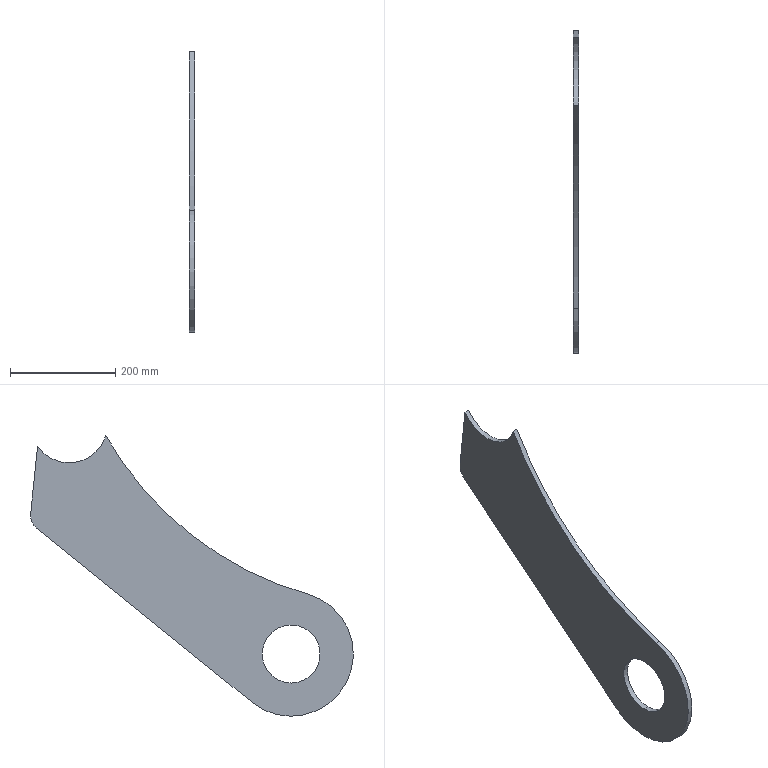Part | SolidWorks | features Extrusion 1 | 1 solid | 10 faces | box 10 x 612.332 x 532.004 mm | volume 1222648 mm3 | cylinder 6 | plane 4 | commonest cylinder face diameters 110 x2 60 x1 146 x1 236.039 x1 1284 x1
STEP:
#1=CARTESIAN_POINT('',(10.,206.6,-676.4));
#2=VERTEX_POINT('',#1);
#3=CARTESIAN_POINT('',(10.,206.6,-786.4));
#4=VERTEX_POINT('',#3);
#5=CARTESIAN_POINT('',(10.,206.6,-731.4));
#6=DIRECTION('',(1.,0.,0.));
#7=DIRECTION('',(0.,0.,-1.));
#8=AXIS2_PLACEMENT_3D('',#5,#6,#7);
#9=CIRCLE('',#8,55.);
#10=EDGE_CURVE('',#2,#4,#9,.T.);
#11=ORIENTED_EDGE('',*,*,#10,.T.);
#12=CARTESIAN_POINT('',(0.,206.6,-786.4));
#13=VERTEX_POINT('',#12);
#14=CARTESIAN_POINT('',(10.,206.6,-786.4));
#15=DIRECTION('',(-1.,0.,0.));
#16=VECTOR('',#15,1000.);
#17=LINE('',#14,#16);
#18=EDGE_CURVE('',#4,#13,#17,.T.);
#19=ORIENTED_EDGE('',*,*,#18,.T.);
#20=CARTESIAN_POINT('',(0.,206.6,-676.4));
#21=VERTEX_POINT('',#20);
#22=CARTESIAN_POINT('',(0.,206.6,-731.4));
#23=DIRECTION('',(1.,0.,0.));
#24=DIRECTION('',(0.,0.,-1.));
#25=AXIS2_PLACEMENT_3D('',#22,#23,#24);
#26=CIRCLE('',#25,55.);
#27=EDGE_CURVE('',#21,#13,#26,.T.);
#28=ORIENTED_EDGE('',*,*,#27,.F.);
#29=CARTESIAN_POINT('',(10.,206.6,-676.4));
#30=DIRECTION('',(-1.,0.,0.));
#31=VECTOR('',#30,1000.);
#32=LINE('',#29,#31);
#33=EDGE_CURVE('',#2,#21,#32,.T.);
#34=ORIENTED_EDGE('',*,*,#33,.F.);
#35=EDGE_LOOP('',(#11,#19,#28,#34));
#36=FACE_OUTER_BOUND('',#35,.T.);
#37=CARTESIAN_POINT('',(10.,206.6,-731.4));
#38=DIRECTION('',(-1.,0.,0.));
#39=DIRECTION('',(0.,0.,1.));
#40=AXIS2_PLACEMENT_3D('',#37,#38,#39);
#41=CYLINDRICAL_SURFACE('',#40,55.);
#42=ADVANCED_FACE('',(#36),#41,.F.);
#43=CARTESIAN_POINT('',(10.,687.7,-337.625));
#44=VERTEX_POINT('',#43);
#45=CARTESIAN_POINT('',(10.,558.043,-317.415));
#46=VERTEX_POINT('',#45);
#47=CARTESIAN_POINT('',(10.,627.8,-295.9));
#48=DIRECTION('',(-1.,0.,0.));
#49=DIRECTION('',(0.,0.,-1.));
#50=AXIS2_PLACEMENT_3D('',#47,#48,#49);
#51=CIRCLE('',#50,73.);
#52=EDGE_CURVE('',#44,#46,#51,.T.);
#53=ORIENTED_EDGE('',*,*,#52,.T.);
#54=CARTESIAN_POINT('',(10.,174.518,-617.825));
#55=VERTEX_POINT('',#54);
#56=CARTESIAN_POINT('',(10.,0.,0.));
#57=DIRECTION('',(-1.,0.,0.));
#58=DIRECTION('',(0.,0.,-1.));
#59=AXIS2_PLACEMENT_3D('',#56,#57,#58);
#60=CIRCLE('',#59,642.);
#61=EDGE_CURVE('',#46,#55,#60,.T.);
#62=ORIENTED_EDGE('',*,*,#61,.T.);
#63=CARTESIAN_POINT('',(10.,280.803,-823.175));
#64=VERTEX_POINT('',#63);
#65=CARTESIAN_POINT('',(10.,206.6,-731.4));
#66=DIRECTION('',(1.,0.,0.));
#67=DIRECTION('',(0.,0.,-1.));
#68=AXIS2_PLACEMENT_3D('',#65,#66,#67);
#69=CIRCLE('',#68,118.019);
#70=EDGE_CURVE('',#55,#64,#69,.T.);
#71=ORIENTED_EDGE('',*,*,#70,.T.);
#72=CARTESIAN_POINT('',(10.,689.774,-492.508));
#73=VERTEX_POINT('',#72);
#74=CARTESIAN_POINT('',(10.,689.774,-492.508));
#75=DIRECTION('',(0.,0.7776,0.6287));
#76=VECTOR('',#75,1000.);
#77=LINE('',#74,#76);
#78=EDGE_CURVE('',#64,#73,#77,.T.);
#79=ORIENTED_EDGE('',*,*,#78,.T.);
#80=CARTESIAN_POINT('',(10.,700.759,-466.147));
#81=VERTEX_POINT('',#80);
#82=CARTESIAN_POINT('',(10.,670.912,-469.18));
#83=DIRECTION('',(1.,0.,0.));
#84=DIRECTION('',(0.,0.,1.));
#85=AXIS2_PLACEMENT_3D('',#82,#83,#84);
#86=CIRCLE('',#85,30.);
#87=EDGE_CURVE('',#73,#81,#86,.T.);
#88=ORIENTED_EDGE('',*,*,#87,.T.);
#89=CARTESIAN_POINT('',(10.,687.7,-337.625));
#90=DIRECTION('',(0.,-0.1011,0.9949));
#91=VECTOR('',#90,1000.);
#92=LINE('',#89,#91);
#93=EDGE_CURVE('',#81,#44,#92,.T.);
#94=ORIENTED_EDGE('',*,*,#93,.T.);
#95=EDGE_LOOP('',(#53,#62,#71,#79,#88,#94));
#96=FACE_OUTER_BOUND('',#95,.T.);
#97=ORIENTED_EDGE('',*,*,#10,.F.);
#98=CARTESIAN_POINT('',(10.,206.6,-731.4));
#99=DIRECTION('',(1.,0.,0.));
#100=DIRECTION('',(0.,0.,-1.));
#101=AXIS2_PLACEMENT_3D('',#98,#99,#100);
#102=CIRCLE('',#101,55.);
#103=EDGE_CURVE('',#4,#2,#102,.T.);
#104=ORIENTED_EDGE('',*,*,#103,.F.);
#105=EDGE_LOOP('',(#97,#104));
#106=FACE_BOUND('',#105,.T.);
#107=CARTESIAN_POINT('',(10.,627.8,-295.9));
#108=DIRECTION('',(1.,0.,0.));
#109=DIRECTION('',(0.,0.,-1.));
#110=AXIS2_PLACEMENT_3D('',#107,#108,#109);
#111=PLANE('',#110);
#112=ADVANCED_FACE('',(#96,#106),#111,.T.);
#113=CARTESIAN_POINT('',(0.,687.7,-337.625));
#114=VERTEX_POINT('',#113);
#115=CARTESIAN_POINT('',(0.,558.043,-317.415));
#116=VERTEX_POINT('',#115);
#117=CARTESIAN_POINT('',(0.,627.8,-295.9));
#118=DIRECTION('',(-1.,0.,0.));
#119=DIRECTION('',(0.,0.,-1.));
#120=AXIS2_PLACEMENT_3D('',#117,#118,#119);
#121=CIRCLE('',#120,73.);
#122=EDGE_CURVE('',#114,#116,#121,.T.);
#123=ORIENTED_EDGE('',*,*,#122,.F.);
#124=CARTESIAN_POINT('',(0.,700.759,-466.147));
#125=VERTEX_POINT('',#124);
#126=CARTESIAN_POINT('',(0.,687.7,-337.625));
#127=DIRECTION('',(0.,-0.1011,0.9949));
#128=VECTOR('',#127,1000.);
#129=LINE('',#126,#128);
#130=EDGE_CURVE('',#125,#114,#129,.T.);
#131=ORIENTED_EDGE('',*,*,#130,.F.);
#132=CARTESIAN_POINT('',(0.,689.774,-492.508));
#133=VERTEX_POINT('',#132);
#134=CARTESIAN_POINT('',(0.,670.912,-469.18));
#135=DIRECTION('',(1.,0.,0.));
#136=DIRECTION('',(0.,0.,1.));
#137=AXIS2_PLACEMENT_3D('',#134,#135,#136);
#138=CIRCLE('',#137,30.);
#139=EDGE_CURVE('',#133,#125,#138,.T.);
#140=ORIENTED_EDGE('',*,*,#139,.F.);
#141=CARTESIAN_POINT('',(0.,280.803,-823.175));
#142=VERTEX_POINT('',#141);
#143=CARTESIAN_POINT('',(0.,689.774,-492.508));
#144=DIRECTION('',(0.,0.7776,0.6287));
#145=VECTOR('',#144,1000.);
#146=LINE('',#143,#145);
#147=EDGE_CURVE('',#142,#133,#146,.T.);
#148=ORIENTED_EDGE('',*,*,#147,.F.);
#149=CARTESIAN_POINT('',(0.,174.518,-617.825));
#150=VERTEX_POINT('',#149);
#151=CARTESIAN_POINT('',(0.,206.6,-731.4));
#152=DIRECTION('',(1.,0.,0.));
#153=DIRECTION('',(0.,0.,-1.));
#154=AXIS2_PLACEMENT_3D('',#151,#152,#153);
#155=CIRCLE('',#154,118.019);
#156=EDGE_CURVE('',#150,#142,#155,.T.);
#157=ORIENTED_EDGE('',*,*,#156,.F.);
#158=CARTESIAN_POINT('',(0.,0.,0.));
#159=DIRECTION('',(-1.,0.,0.));
#160=DIRECTION('',(0.,0.,-1.));
#161=AXIS2_PLACEMENT_3D('',#158,#159,#160);
#162=CIRCLE('',#161,642.);
#163=EDGE_CURVE('',#116,#150,#162,.T.);
#164=ORIENTED_EDGE('',*,*,#163,.F.);
#165=EDGE_LOOP('',(#123,#131,#140,#148,#157,#164));
#166=FACE_OUTER_BOUND('',#165,.T.);
#167=ORIENTED_EDGE('',*,*,#27,.T.);
#168=CARTESIAN_POINT('',(0.,206.6,-731.4));
#169=DIRECTION('',(1.,0.,0.));
#170=DIRECTION('',(0.,0.,-1.));
#171=AXIS2_PLACEMENT_3D('',#168,#169,#170);
#172=CIRCLE('',#171,55.);
#173=EDGE_CURVE('',#13,#21,#172,.T.);
#174=ORIENTED_EDGE('',*,*,#173,.T.);
#175=EDGE_LOOP('',(#167,#174));
#176=FACE_BOUND('',#175,.T.);
#177=CARTESIAN_POINT('',(0.,627.8,-295.9));
#178=DIRECTION('',(1.,0.,0.));
#179=DIRECTION('',(0.,0.,-1.));
#180=AXIS2_PLACEMENT_3D('',#177,#178,#179);
#181=PLANE('',#180);
#182=ADVANCED_FACE('',(#166,#176),#181,.F.);
#183=ORIENTED_EDGE('',*,*,#122,.T.);
#184=CARTESIAN_POINT('',(10.,558.043,-317.415));
#185=DIRECTION('',(-1.,0.,0.));
#186=VECTOR('',#185,1000.);
#187=LINE('',#184,#186);
#188=EDGE_CURVE('',#46,#116,#187,.T.);
#189=ORIENTED_EDGE('',*,*,#188,.F.);
#190=ORIENTED_EDGE('',*,*,#52,.F.);
#191=CARTESIAN_POINT('',(10.,687.7,-337.625));
#192=DIRECTION('',(-1.,0.,0.));
#193=VECTOR('',#192,1000.);
#194=LINE('',#191,#193);
#195=EDGE_CURVE('',#44,#114,#194,.T.);
#196=ORIENTED_EDGE('',*,*,#195,.T.);
#197=EDGE_LOOP('',(#183,#189,#190,#196));
#198=FACE_OUTER_BOUND('',#197,.T.);
#199=CARTESIAN_POINT('',(10.,627.8,-295.9));
#200=DIRECTION('',(-1.,0.,0.));
#201=DIRECTION('',(0.,0.,1.));
#202=AXIS2_PLACEMENT_3D('',#199,#200,#201);
#203=CYLINDRICAL_SURFACE('',#202,73.);
#204=ADVANCED_FACE('',(#198),#203,.F.);
#205=ORIENTED_EDGE('',*,*,#163,.T.);
#206=CARTESIAN_POINT('',(10.,174.518,-617.825));
#207=DIRECTION('',(-1.,0.,0.));
#208=VECTOR('',#207,1000.);
#209=LINE('',#206,#208);
#210=EDGE_CURVE('',#55,#150,#209,.T.);
#211=ORIENTED_EDGE('',*,*,#210,.F.);
#212=ORIENTED_EDGE('',*,*,#61,.F.);
#213=ORIENTED_EDGE('',*,*,#188,.T.);
#214=EDGE_LOOP('',(#205,#211,#212,#213));
#215=FACE_OUTER_BOUND('',#214,.T.);
#216=CARTESIAN_POINT('',(10.,0.,0.));
#217=DIRECTION('',(-1.,0.,0.));
#218=DIRECTION('',(0.,0.,1.));
#219=AXIS2_PLACEMENT_3D('',#216,#217,#218);
#220=CYLINDRICAL_SURFACE('',#219,642.);
#221=ADVANCED_FACE('',(#215),#220,.F.);
#222=ORIENTED_EDGE('',*,*,#156,.T.);
#223=CARTESIAN_POINT('',(10.,280.803,-823.175));
#224=DIRECTION('',(-1.,0.,0.));
#225=VECTOR('',#224,1000.);
#226=LINE('',#223,#225);
#227=EDGE_CURVE('',#64,#142,#226,.T.);
#228=ORIENTED_EDGE('',*,*,#227,.F.);
#229=ORIENTED_EDGE('',*,*,#70,.F.);
#230=ORIENTED_EDGE('',*,*,#210,.T.);
#231=EDGE_LOOP('',(#222,#228,#229,#230));
#232=FACE_OUTER_BOUND('',#231,.T.);
#233=CARTESIAN_POINT('',(10.,206.6,-731.4));
#234=DIRECTION('',(-1.,0.,0.));
#235=DIRECTION('',(0.,0.,1.));
#236=AXIS2_PLACEMENT_3D('',#233,#234,#235);
#237=CYLINDRICAL_SURFACE('',#236,118.019);
#238=ADVANCED_FACE('',(#232),#237,.T.);
#239=ORIENTED_EDGE('',*,*,#147,.T.);
#240=CARTESIAN_POINT('',(10.,689.774,-492.508));
#241=DIRECTION('',(-1.,0.,0.));
#242=VECTOR('',#241,1000.);
#243=LINE('',#240,#242);
#244=EDGE_CURVE('',#73,#133,#243,.T.);
#245=ORIENTED_EDGE('',*,*,#244,.F.);
#246=ORIENTED_EDGE('',*,*,#78,.F.);
#247=ORIENTED_EDGE('',*,*,#227,.T.);
#248=EDGE_LOOP('',(#239,#245,#246,#247));
#249=FACE_OUTER_BOUND('',#248,.T.);
#250=CARTESIAN_POINT('',(10.,689.774,-492.508));
#251=DIRECTION('',(0.,-0.6287,0.7776));
#252=DIRECTION('',(0.,-0.7776,-0.6287));
#253=AXIS2_PLACEMENT_3D('',#250,#251,#252);
#254=PLANE('',#253);
#255=ADVANCED_FACE('',(#249),#254,.F.);
#256=ORIENTED_EDGE('',*,*,#139,.T.);
#257=CARTESIAN_POINT('',(10.,700.759,-466.147));
#258=DIRECTION('',(-1.,0.,0.));
#259=VECTOR('',#258,1000.);
#260=LINE('',#257,#259);
#261=EDGE_CURVE('',#81,#125,#260,.T.);
#262=ORIENTED_EDGE('',*,*,#261,.F.);
#263=ORIENTED_EDGE('',*,*,#87,.F.);
#264=ORIENTED_EDGE('',*,*,#244,.T.);
#265=EDGE_LOOP('',(#256,#262,#263,#264));
#266=FACE_OUTER_BOUND('',#265,.T.);
#267=CARTESIAN_POINT('',(10.,670.912,-469.18));
#268=DIRECTION('',(-1.,0.,0.));
#269=DIRECTION('',(0.,0.,1.));
#270=AXIS2_PLACEMENT_3D('',#267,#268,#269);
#271=CYLINDRICAL_SURFACE('',#270,30.);
#272=ADVANCED_FACE('',(#266),#271,.T.);
#273=ORIENTED_EDGE('',*,*,#130,.T.);
#274=ORIENTED_EDGE('',*,*,#195,.F.);
#275=ORIENTED_EDGE('',*,*,#93,.F.);
#276=ORIENTED_EDGE('',*,*,#261,.T.);
#277=EDGE_LOOP('',(#273,#274,#275,#276));
#278=FACE_OUTER_BOUND('',#277,.T.);
#279=CARTESIAN_POINT('',(10.,687.7,-337.625));
#280=DIRECTION('',(0.,-0.9949,-0.1011));
#281=DIRECTION('',(0.,0.1011,-0.9949));
#282=AXIS2_PLACEMENT_3D('',#279,#280,#281);
#283=PLANE('',#282);
#284=ADVANCED_FACE('',(#278),#283,.F.);
#285=ORIENTED_EDGE('',*,*,#18,.F.);
#286=ORIENTED_EDGE('',*,*,#103,.T.);
#287=ORIENTED_EDGE('',*,*,#33,.T.);
#288=ORIENTED_EDGE('',*,*,#173,.F.);
#289=EDGE_LOOP('',(#285,#286,#287,#288));
#290=FACE_OUTER_BOUND('',#289,.T.);
#291=CARTESIAN_POINT('',(10.,206.6,-731.4));
#292=DIRECTION('',(-1.,0.,0.));
#293=DIRECTION('',(0.,0.,1.));
#294=AXIS2_PLACEMENT_3D('',#291,#292,#293);
#295=CYLINDRICAL_SURFACE('',#294,55.);
#296=ADVANCED_FACE('',(#290),#295,.F.);
#297=CLOSED_SHELL('',(#42,#112,#182,#204,#221,#238,#255,#272,#284,#296));
#298=MANIFOLD_SOLID_BREP('',#297);
#299=CARTESIAN_POINT('',(0.,0.,0.));
#300=DIRECTION('',(0.,0.,1.));
#301=DIRECTION('',(1.,0.,0.));
#302=AXIS2_PLACEMENT_3D('',#299,#300,#301);
#303=(LENGTH_UNIT()NAMED_UNIT(*)SI_UNIT(.MILLI.,.METRE.));
#304=UNCERTAINTY_MEASURE_WITH_UNIT(LENGTH_MEASURE(0.00001),#303,'','');
#305=(NAMED_UNIT(*)PLANE_ANGLE_UNIT()SI_UNIT($,.RADIAN.));
#306=(NAMED_UNIT(*)SI_UNIT($,.STERADIAN.)SOLID_ANGLE_UNIT());
#307=(GEOMETRIC_REPRESENTATION_CONTEXT(3)GLOBAL_UNCERTAINTY_ASSIGNED_CONTEXT((#304))GLOBAL_UNIT_ASSIGNED_CONTEXT((#303,#305,#306))REPRESENTATION_CONTEXT('',''));
#308=ADVANCED_BREP_SHAPE_REPRESENTATION('',(#298,#302),#307);